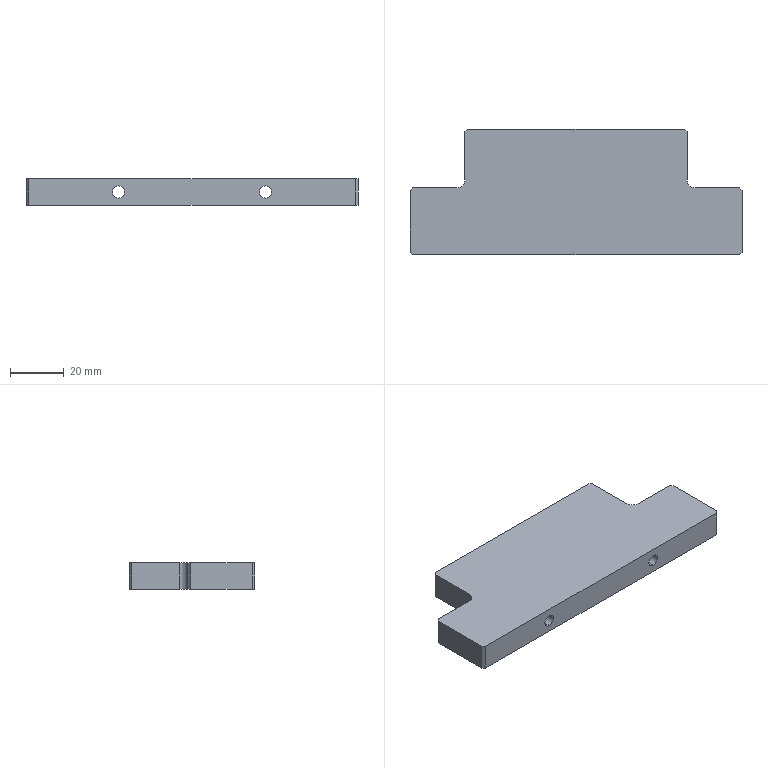Part | STEP file | 1 solid | 44 faces | box 124 x 47 x 10 mm | volume 44873 mm3 | cylinder 18 | plane 18 | cone 8 | commonest cylinder face diameters 2.5 x8 4.5 x4 8 x4 6 x2